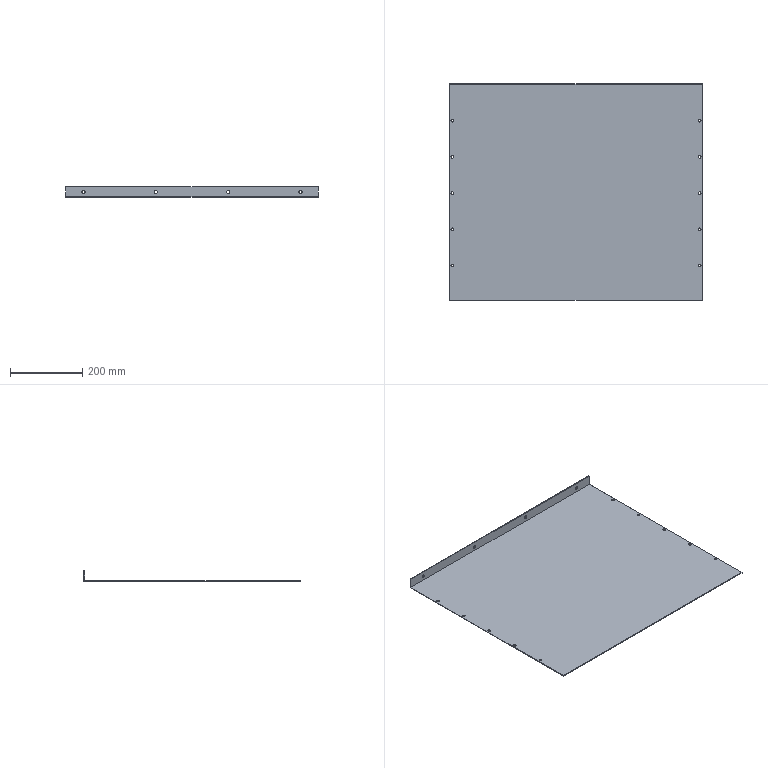Part | SolidWorks | features BaseBody 1 | 1 solid | 36 faces | box 699 x 599 x 30 mm | volume 1093155 mm3 | cylinder 28 | plane 8 | commonest cylinder face diameters 7.2 x20 9 x8
STEP:
#1=CARTESIAN_POINT('',(201.346,-3540.973,1409.971));
#2=VERTEX_POINT('',#1);
#3=CARTESIAN_POINT('',(208.546,-3540.973,1409.971));
#4=VERTEX_POINT('',#3);
#5=CARTESIAN_POINT('',(204.946,-3540.973,1409.971));
#6=DIRECTION('',(0.,0.,1.));
#7=DIRECTION('',(1.,0.,0.));
#8=AXIS2_PLACEMENT_3D('',#5,#6,#7);
#9=CIRCLE('',#8,3.6);
#10=EDGE_CURVE('',#2,#4,#9,.T.);
#11=ORIENTED_EDGE('',*,*,#10,.F.);
#12=CARTESIAN_POINT('',(201.346,-3540.973,1412.471));
#13=VERTEX_POINT('',#12);
#14=CARTESIAN_POINT('',(201.346,-3540.973,1411.476));
#15=DIRECTION('',(0.,0.,1.));
#16=VECTOR('',#15,1000.);
#17=LINE('',#14,#16);
#18=EDGE_CURVE('',#2,#13,#17,.T.);
#19=ORIENTED_EDGE('',*,*,#18,.T.);
#20=CARTESIAN_POINT('',(208.546,-3540.973,1412.471));
#21=VERTEX_POINT('',#20);
#22=CARTESIAN_POINT('',(204.946,-3540.973,1412.471));
#23=DIRECTION('',(0.,0.,-1.));
#24=DIRECTION('',(1.,0.,0.));
#25=AXIS2_PLACEMENT_3D('',#22,#23,#24);
#26=CIRCLE('',#25,3.6);
#27=EDGE_CURVE('',#21,#13,#26,.T.);
#28=ORIENTED_EDGE('',*,*,#27,.F.);
#29=CARTESIAN_POINT('',(208.546,-3540.973,1411.476));
#30=DIRECTION('',(0.,0.,1.));
#31=VECTOR('',#30,1000.);
#32=LINE('',#29,#31);
#33=EDGE_CURVE('',#4,#21,#32,.T.);
#34=ORIENTED_EDGE('',*,*,#33,.F.);
#35=EDGE_LOOP('',(#11,#19,#28,#34));
#36=FACE_OUTER_BOUND('',#35,.T.);
#37=CARTESIAN_POINT('',(204.946,-3540.973,1411.476));
#38=DIRECTION('',(0.,0.,1.));
#39=DIRECTION('',(1.,0.,0.));
#40=AXIS2_PLACEMENT_3D('',#37,#38,#39);
#41=CYLINDRICAL_SURFACE('',#40,3.6);
#42=ADVANCED_FACE('',(#36),#41,.F.);
#43=CARTESIAN_POINT('',(201.346,-3340.973,1409.971));
#44=VERTEX_POINT('',#43);
#45=CARTESIAN_POINT('',(208.546,-3340.973,1409.971));
#46=VERTEX_POINT('',#45);
#47=CARTESIAN_POINT('',(204.946,-3340.973,1409.971));
#48=DIRECTION('',(0.,0.,1.));
#49=DIRECTION('',(1.,0.,0.));
#50=AXIS2_PLACEMENT_3D('',#47,#48,#49);
#51=CIRCLE('',#50,3.6);
#52=EDGE_CURVE('',#44,#46,#51,.T.);
#53=ORIENTED_EDGE('',*,*,#52,.F.);
#54=CARTESIAN_POINT('',(201.346,-3340.973,1412.471));
#55=VERTEX_POINT('',#54);
#56=CARTESIAN_POINT('',(201.346,-3340.973,1411.476));
#57=DIRECTION('',(0.,0.,1.));
#58=VECTOR('',#57,1000.);
#59=LINE('',#56,#58);
#60=EDGE_CURVE('',#44,#55,#59,.T.);
#61=ORIENTED_EDGE('',*,*,#60,.T.);
#62=CARTESIAN_POINT('',(208.546,-3340.973,1412.471));
#63=VERTEX_POINT('',#62);
#64=CARTESIAN_POINT('',(204.946,-3340.973,1412.471));
#65=DIRECTION('',(0.,0.,-1.));
#66=DIRECTION('',(1.,0.,0.));
#67=AXIS2_PLACEMENT_3D('',#64,#65,#66);
#68=CIRCLE('',#67,3.6);
#69=EDGE_CURVE('',#63,#55,#68,.T.);
#70=ORIENTED_EDGE('',*,*,#69,.F.);
#71=CARTESIAN_POINT('',(208.546,-3340.973,1411.476));
#72=DIRECTION('',(0.,0.,1.));
#73=VECTOR('',#72,1000.);
#74=LINE('',#71,#73);
#75=EDGE_CURVE('',#46,#63,#74,.T.);
#76=ORIENTED_EDGE('',*,*,#75,.F.);
#77=EDGE_LOOP('',(#53,#61,#70,#76));
#78=FACE_OUTER_BOUND('',#77,.T.);
#79=CARTESIAN_POINT('',(204.946,-3340.973,1411.476));
#80=DIRECTION('',(0.,0.,1.));
#81=DIRECTION('',(1.,0.,0.));
#82=AXIS2_PLACEMENT_3D('',#79,#80,#81);
#83=CYLINDRICAL_SURFACE('',#82,3.6);
#84=ADVANCED_FACE('',(#78),#83,.F.);
#85=CARTESIAN_POINT('',(201.346,-3140.973,1409.971));
#86=VERTEX_POINT('',#85);
#87=CARTESIAN_POINT('',(208.546,-3140.973,1409.971));
#88=VERTEX_POINT('',#87);
#89=CARTESIAN_POINT('',(204.946,-3140.973,1409.971));
#90=DIRECTION('',(0.,0.,1.));
#91=DIRECTION('',(1.,0.,0.));
#92=AXIS2_PLACEMENT_3D('',#89,#90,#91);
#93=CIRCLE('',#92,3.6);
#94=EDGE_CURVE('',#86,#88,#93,.T.);
#95=ORIENTED_EDGE('',*,*,#94,.F.);
#96=CARTESIAN_POINT('',(201.346,-3140.973,1412.471));
#97=VERTEX_POINT('',#96);
#98=CARTESIAN_POINT('',(201.346,-3140.973,1411.476));
#99=DIRECTION('',(0.,0.,1.));
#100=VECTOR('',#99,1000.);
#101=LINE('',#98,#100);
#102=EDGE_CURVE('',#86,#97,#101,.T.);
#103=ORIENTED_EDGE('',*,*,#102,.T.);
#104=CARTESIAN_POINT('',(208.546,-3140.973,1412.471));
#105=VERTEX_POINT('',#104);
#106=CARTESIAN_POINT('',(204.946,-3140.973,1412.471));
#107=DIRECTION('',(0.,0.,-1.));
#108=DIRECTION('',(1.,0.,0.));
#109=AXIS2_PLACEMENT_3D('',#106,#107,#108);
#110=CIRCLE('',#109,3.6);
#111=EDGE_CURVE('',#105,#97,#110,.T.);
#112=ORIENTED_EDGE('',*,*,#111,.F.);
#113=CARTESIAN_POINT('',(208.546,-3140.973,1411.476));
#114=DIRECTION('',(0.,0.,1.));
#115=VECTOR('',#114,1000.);
#116=LINE('',#113,#115);
#117=EDGE_CURVE('',#88,#105,#116,.T.);
#118=ORIENTED_EDGE('',*,*,#117,.F.);
#119=EDGE_LOOP('',(#95,#103,#112,#118));
#120=FACE_OUTER_BOUND('',#119,.T.);
#121=CARTESIAN_POINT('',(204.946,-3140.973,1411.476));
#122=DIRECTION('',(0.,0.,1.));
#123=DIRECTION('',(1.,0.,0.));
#124=AXIS2_PLACEMENT_3D('',#121,#122,#123);
#125=CYLINDRICAL_SURFACE('',#124,3.6);
#126=ADVANCED_FACE('',(#120),#125,.F.);
#127=CARTESIAN_POINT('',(892.546,-3440.973,1412.471));
#128=VERTEX_POINT('',#127);
#129=CARTESIAN_POINT('',(885.346,-3440.973,1412.471));
#130=VERTEX_POINT('',#129);
#131=CARTESIAN_POINT('',(888.946,-3440.973,1412.471));
#132=DIRECTION('',(0.,0.,-1.));
#133=DIRECTION('',(-1.,0.,0.));
#134=AXIS2_PLACEMENT_3D('',#131,#132,#133);
#135=CIRCLE('',#134,3.6);
#136=EDGE_CURVE('',#128,#130,#135,.T.);
#137=ORIENTED_EDGE('',*,*,#136,.F.);
#138=CARTESIAN_POINT('',(892.546,-3440.973,1409.971));
#139=VERTEX_POINT('',#138);
#140=CARTESIAN_POINT('',(892.546,-3440.973,1411.476));
#141=DIRECTION('',(0.,0.,-1.));
#142=VECTOR('',#141,1000.);
#143=LINE('',#140,#142);
#144=EDGE_CURVE('',#128,#139,#143,.T.);
#145=ORIENTED_EDGE('',*,*,#144,.T.);
#146=CARTESIAN_POINT('',(885.346,-3440.973,1409.971));
#147=VERTEX_POINT('',#146);
#148=CARTESIAN_POINT('',(888.946,-3440.973,1409.971));
#149=DIRECTION('',(0.,0.,1.));
#150=DIRECTION('',(-1.,0.,0.));
#151=AXIS2_PLACEMENT_3D('',#148,#149,#150);
#152=CIRCLE('',#151,3.6);
#153=EDGE_CURVE('',#147,#139,#152,.T.);
#154=ORIENTED_EDGE('',*,*,#153,.F.);
#155=CARTESIAN_POINT('',(885.346,-3440.973,1411.476));
#156=DIRECTION('',(0.,0.,-1.));
#157=VECTOR('',#156,1000.);
#158=LINE('',#155,#157);
#159=EDGE_CURVE('',#130,#147,#158,.T.);
#160=ORIENTED_EDGE('',*,*,#159,.F.);
#161=EDGE_LOOP('',(#137,#145,#154,#160));
#162=FACE_OUTER_BOUND('',#161,.T.);
#163=CARTESIAN_POINT('',(888.946,-3440.973,1411.476));
#164=DIRECTION('',(0.,0.,-1.));
#165=DIRECTION('',(-1.,0.,0.));
#166=AXIS2_PLACEMENT_3D('',#163,#164,#165);
#167=CYLINDRICAL_SURFACE('',#166,3.6);
#168=ADVANCED_FACE('',(#162),#167,.F.);
#169=CARTESIAN_POINT('',(892.546,-3240.973,1412.471));
#170=VERTEX_POINT('',#169);
#171=CARTESIAN_POINT('',(885.346,-3240.973,1412.471));
#172=VERTEX_POINT('',#171);
#173=CARTESIAN_POINT('',(888.946,-3240.973,1412.471));
#174=DIRECTION('',(0.,0.,-1.));
#175=DIRECTION('',(-1.,0.,0.));
#176=AXIS2_PLACEMENT_3D('',#173,#174,#175);
#177=CIRCLE('',#176,3.6);
#178=EDGE_CURVE('',#170,#172,#177,.T.);
#179=ORIENTED_EDGE('',*,*,#178,.F.);
#180=CARTESIAN_POINT('',(892.546,-3240.973,1409.971));
#181=VERTEX_POINT('',#180);
#182=CARTESIAN_POINT('',(892.546,-3240.973,1411.476));
#183=DIRECTION('',(0.,0.,-1.));
#184=VECTOR('',#183,1000.);
#185=LINE('',#182,#184);
#186=EDGE_CURVE('',#170,#181,#185,.T.);
#187=ORIENTED_EDGE('',*,*,#186,.T.);
#188=CARTESIAN_POINT('',(885.346,-3240.973,1409.971));
#189=VERTEX_POINT('',#188);
#190=CARTESIAN_POINT('',(888.946,-3240.973,1409.971));
#191=DIRECTION('',(0.,0.,1.));
#192=DIRECTION('',(-1.,0.,0.));
#193=AXIS2_PLACEMENT_3D('',#190,#191,#192);
#194=CIRCLE('',#193,3.6);
#195=EDGE_CURVE('',#189,#181,#194,.T.);
#196=ORIENTED_EDGE('',*,*,#195,.F.);
#197=CARTESIAN_POINT('',(885.346,-3240.973,1411.476));
#198=DIRECTION('',(0.,0.,-1.));
#199=VECTOR('',#198,1000.);
#200=LINE('',#197,#199);
#201=EDGE_CURVE('',#172,#189,#200,.T.);
#202=ORIENTED_EDGE('',*,*,#201,.F.);
#203=EDGE_LOOP('',(#179,#187,#196,#202));
#204=FACE_OUTER_BOUND('',#203,.T.);
#205=CARTESIAN_POINT('',(888.946,-3240.973,1411.476));
#206=DIRECTION('',(0.,0.,-1.));
#207=DIRECTION('',(-1.,0.,0.));
#208=AXIS2_PLACEMENT_3D('',#205,#206,#207);
#209=CYLINDRICAL_SURFACE('',#208,3.6);
#210=ADVANCED_FACE('',(#204),#209,.F.);
#211=CARTESIAN_POINT('',(892.546,-3140.973,1412.471));
#212=VERTEX_POINT('',#211);
#213=CARTESIAN_POINT('',(885.346,-3140.973,1412.471));
#214=VERTEX_POINT('',#213);
#215=CARTESIAN_POINT('',(888.946,-3140.973,1412.471));
#216=DIRECTION('',(0.,0.,-1.));
#217=DIRECTION('',(-1.,0.,0.));
#218=AXIS2_PLACEMENT_3D('',#215,#216,#217);
#219=CIRCLE('',#218,3.6);
#220=EDGE_CURVE('',#212,#214,#219,.T.);
#221=ORIENTED_EDGE('',*,*,#220,.F.);
#222=CARTESIAN_POINT('',(892.546,-3140.973,1409.971));
#223=VERTEX_POINT('',#222);
#224=CARTESIAN_POINT('',(892.546,-3140.973,1411.476));
#225=DIRECTION('',(0.,0.,-1.));
#226=VECTOR('',#225,1000.);
#227=LINE('',#224,#226);
#228=EDGE_CURVE('',#212,#223,#227,.T.);
#229=ORIENTED_EDGE('',*,*,#228,.T.);
#230=CARTESIAN_POINT('',(885.346,-3140.973,1409.971));
#231=VERTEX_POINT('',#230);
#232=CARTESIAN_POINT('',(888.946,-3140.973,1409.971));
#233=DIRECTION('',(0.,0.,1.));
#234=DIRECTION('',(-1.,0.,0.));
#235=AXIS2_PLACEMENT_3D('',#232,#233,#234);
#236=CIRCLE('',#235,3.6);
#237=EDGE_CURVE('',#231,#223,#236,.T.);
#238=ORIENTED_EDGE('',*,*,#237,.F.);
#239=CARTESIAN_POINT('',(885.346,-3140.973,1411.476));
#240=DIRECTION('',(0.,0.,-1.));
#241=VECTOR('',#240,1000.);
#242=LINE('',#239,#241);
#243=EDGE_CURVE('',#214,#231,#242,.T.);
#244=ORIENTED_EDGE('',*,*,#243,.F.);
#245=EDGE_LOOP('',(#221,#229,#238,#244));
#246=FACE_OUTER_BOUND('',#245,.T.);
#247=CARTESIAN_POINT('',(888.946,-3140.973,1411.476));
#248=DIRECTION('',(0.,0.,-1.));
#249=DIRECTION('',(-1.,0.,0.));
#250=AXIS2_PLACEMENT_3D('',#247,#248,#249);
#251=CYLINDRICAL_SURFACE('',#250,3.6);
#252=ADVANCED_FACE('',(#246),#251,.F.);
#253=CARTESIAN_POINT('',(892.546,-3340.973,1412.471));
#254=VERTEX_POINT('',#253);
#255=CARTESIAN_POINT('',(885.346,-3340.973,1412.471));
#256=VERTEX_POINT('',#255);
#257=CARTESIAN_POINT('',(888.946,-3340.973,1412.471));
#258=DIRECTION('',(0.,0.,-1.));
#259=DIRECTION('',(-1.,0.,0.));
#260=AXIS2_PLACEMENT_3D('',#257,#258,#259);
#261=CIRCLE('',#260,3.6);
#262=EDGE_CURVE('',#254,#256,#261,.T.);
#263=ORIENTED_EDGE('',*,*,#262,.F.);
#264=CARTESIAN_POINT('',(892.546,-3340.973,1409.971));
#265=VERTEX_POINT('',#264);
#266=CARTESIAN_POINT('',(892.546,-3340.973,1411.476));
#267=DIRECTION('',(0.,0.,-1.));
#268=VECTOR('',#267,1000.);
#269=LINE('',#266,#268);
#270=EDGE_CURVE('',#254,#265,#269,.T.);
#271=ORIENTED_EDGE('',*,*,#270,.T.);
#272=CARTESIAN_POINT('',(885.346,-3340.973,1409.971));
#273=VERTEX_POINT('',#272);
#274=CARTESIAN_POINT('',(888.946,-3340.973,1409.971));
#275=DIRECTION('',(0.,0.,1.));
#276=DIRECTION('',(-1.,0.,0.));
#277=AXIS2_PLACEMENT_3D('',#274,#275,#276);
#278=CIRCLE('',#277,3.6);
#279=EDGE_CURVE('',#273,#265,#278,.T.);
#280=ORIENTED_EDGE('',*,*,#279,.F.);
#281=CARTESIAN_POINT('',(885.346,-3340.973,1411.476));
#282=DIRECTION('',(0.,0.,-1.));
#283=VECTOR('',#282,1000.);
#284=LINE('',#281,#283);
#285=EDGE_CURVE('',#256,#273,#284,.T.);
#286=ORIENTED_EDGE('',*,*,#285,.F.);
#287=EDGE_LOOP('',(#263,#271,#280,#286));
#288=FACE_OUTER_BOUND('',#287,.T.);
#289=CARTESIAN_POINT('',(888.946,-3340.973,1411.476));
#290=DIRECTION('',(0.,0.,-1.));
#291=DIRECTION('',(-1.,0.,0.));
#292=AXIS2_PLACEMENT_3D('',#289,#290,#291);
#293=CYLINDRICAL_SURFACE('',#292,3.6);
#294=ADVANCED_FACE('',(#288),#293,.F.);
#295=CARTESIAN_POINT('',(892.546,-3540.973,1412.471));
#296=VERTEX_POINT('',#295);
#297=CARTESIAN_POINT('',(885.346,-3540.973,1412.471));
#298=VERTEX_POINT('',#297);
#299=CARTESIAN_POINT('',(888.946,-3540.973,1412.471));
#300=DIRECTION('',(0.,0.,-1.));
#301=DIRECTION('',(-1.,0.,0.));
#302=AXIS2_PLACEMENT_3D('',#299,#300,#301);
#303=CIRCLE('',#302,3.6);
#304=EDGE_CURVE('',#296,#298,#303,.T.);
#305=ORIENTED_EDGE('',*,*,#304,.F.);
#306=CARTESIAN_POINT('',(892.546,-3540.973,1409.971));
#307=VERTEX_POINT('',#306);
#308=CARTESIAN_POINT('',(892.546,-3540.973,1411.476));
#309=DIRECTION('',(0.,0.,-1.));
#310=VECTOR('',#309,1000.);
#311=LINE('',#308,#310);
#312=EDGE_CURVE('',#296,#307,#311,.T.);
#313=ORIENTED_EDGE('',*,*,#312,.T.);
#314=CARTESIAN_POINT('',(885.346,-3540.973,1409.971));
#315=VERTEX_POINT('',#314);
#316=CARTESIAN_POINT('',(888.946,-3540.973,1409.971));
#317=DIRECTION('',(0.,0.,1.));
#318=DIRECTION('',(-1.,0.,0.));
#319=AXIS2_PLACEMENT_3D('',#316,#317,#318);
#320=CIRCLE('',#319,3.6);
#321=EDGE_CURVE('',#315,#307,#320,.T.);
#322=ORIENTED_EDGE('',*,*,#321,.F.);
#323=CARTESIAN_POINT('',(885.346,-3540.973,1411.476));
#324=DIRECTION('',(0.,0.,-1.));
#325=VECTOR('',#324,1000.);
#326=LINE('',#323,#325);
#327=EDGE_CURVE('',#298,#315,#326,.T.);
#328=ORIENTED_EDGE('',*,*,#327,.F.);
#329=EDGE_LOOP('',(#305,#313,#322,#328));
#330=FACE_OUTER_BOUND('',#329,.T.);
#331=CARTESIAN_POINT('',(888.946,-3540.973,1411.476));
#332=DIRECTION('',(0.,0.,-1.));
#333=DIRECTION('',(-1.,0.,0.));
#334=AXIS2_PLACEMENT_3D('',#331,#332,#333);
#335=CYLINDRICAL_SURFACE('',#334,3.6);
#336=ADVANCED_FACE('',(#330),#335,.F.);
#337=CARTESIAN_POINT('',(201.346,-3240.973,1409.971));
#338=VERTEX_POINT('',#337);
#339=CARTESIAN_POINT('',(208.546,-3240.973,1409.971));
#340=VERTEX_POINT('',#339);
#341=CARTESIAN_POINT('',(204.946,-3240.973,1409.971));
#342=DIRECTION('',(0.,0.,1.));
#343=DIRECTION('',(1.,0.,0.));
#344=AXIS2_PLACEMENT_3D('',#341,#342,#343);
#345=CIRCLE('',#344,3.6);
#346=EDGE_CURVE('',#338,#340,#345,.T.);
#347=ORIENTED_EDGE('',*,*,#346,.F.);
#348=CARTESIAN_POINT('',(201.346,-3240.973,1412.471));
#349=VERTEX_POINT('',#348);
#350=CARTESIAN_POINT('',(201.346,-3240.973,1411.476));
#351=DIRECTION('',(0.,0.,1.));
#352=VECTOR('',#351,1000.);
#353=LINE('',#350,#352);
#354=EDGE_CURVE('',#338,#349,#353,.T.);
#355=ORIENTED_EDGE('',*,*,#354,.T.);
#356=CARTESIAN_POINT('',(208.546,-3240.973,1412.471));
#357=VERTEX_POINT('',#356);
#358=CARTESIAN_POINT('',(204.946,-3240.973,1412.471));
#359=DIRECTION('',(0.,0.,-1.));
#360=DIRECTION('',(1.,0.,0.));
#361=AXIS2_PLACEMENT_3D('',#358,#359,#360);
#362=CIRCLE('',#361,3.6);
#363=EDGE_CURVE('',#357,#349,#362,.T.);
#364=ORIENTED_EDGE('',*,*,#363,.F.);
#365=CARTESIAN_POINT('',(208.546,-3240.973,1411.476));
#366=DIRECTION('',(0.,0.,1.));
#367=VECTOR('',#366,1000.);
#368=LINE('',#365,#367);
#369=EDGE_CURVE('',#340,#357,#368,.T.);
#370=ORIENTED_EDGE('',*,*,#369,.F.);
#371=EDGE_LOOP('',(#347,#355,#364,#370));
#372=FACE_OUTER_BOUND('',#371,.T.);
#373=CARTESIAN_POINT('',(204.946,-3240.973,1411.476));
#374=DIRECTION('',(0.,0.,1.));
#375=DIRECTION('',(1.,0.,0.));
#376=AXIS2_PLACEMENT_3D('',#373,#374,#375);
#377=CYLINDRICAL_SURFACE('',#376,3.6);
#378=ADVANCED_FACE('',(#372),#377,.F.);
#379=CARTESIAN_POINT('',(201.346,-3440.973,1409.971));
#380=VERTEX_POINT('',#379);
#381=CARTESIAN_POINT('',(208.546,-3440.973,1409.971));
#382=VERTEX_POINT('',#381);
#383=CARTESIAN_POINT('',(204.946,-3440.973,1409.971));
#384=DIRECTION('',(0.,0.,1.));
#385=DIRECTION('',(1.,0.,0.));
#386=AXIS2_PLACEMENT_3D('',#383,#384,#385);
#387=CIRCLE('',#386,3.6);
#388=EDGE_CURVE('',#380,#382,#387,.T.);
#389=ORIENTED_EDGE('',*,*,#388,.F.);
#390=CARTESIAN_POINT('',(201.346,-3440.973,1412.471));
#391=VERTEX_POINT('',#390);
#392=CARTESIAN_POINT('',(201.346,-3440.973,1411.476));
#393=DIRECTION('',(0.,0.,1.));
#394=VECTOR('',#393,1000.);
#395=LINE('',#392,#394);
#396=EDGE_CURVE('',#380,#391,#395,.T.);
#397=ORIENTED_EDGE('',*,*,#396,.T.);
#398=CARTESIAN_POINT('',(208.546,-3440.973,1412.471));
#399=VERTEX_POINT('',#398);
#400=CARTESIAN_POINT('',(204.946,-3440.973,1412.471));
#401=DIRECTION('',(0.,0.,-1.));
#402=DIRECTION('',(1.,0.,0.));
#403=AXIS2_PLACEMENT_3D('',#400,#401,#402);
#404=CIRCLE('',#403,3.6);
#405=EDGE_CURVE('',#399,#391,#404,.T.);
#406=ORIENTED_EDGE('',*,*,#405,.F.);
#407=CARTESIAN_POINT('',(208.546,-3440.973,1411.476));
#408=DIRECTION('',(0.,0.,1.));
#409=VECTOR('',#408,1000.);
#410=LINE('',#407,#409);
#411=EDGE_CURVE('',#382,#399,#410,.T.);
#412=ORIENTED_EDGE('',*,*,#411,.F.);
#413=EDGE_LOOP('',(#389,#397,#406,#412));
#414=FACE_OUTER_BOUND('',#413,.T.);
#415=CARTESIAN_POINT('',(204.946,-3440.973,1411.476));
#416=DIRECTION('',(0.,0.,1.));
#417=DIRECTION('',(1.,0.,0.));
#418=AXIS2_PLACEMENT_3D('',#415,#416,#417);
#419=CYLINDRICAL_SURFACE('',#418,3.6);
#420=ADVANCED_FACE('',(#414),#419,.F.);
#421=CARTESIAN_POINT('',(446.946,-3040.973,1420.471));
#422=VERTEX_POINT('',#421);
#423=CARTESIAN_POINT('',(446.946,-3040.973,1429.471));
#424=VERTEX_POINT('',#423);
#425=CARTESIAN_POINT('',(446.946,-3040.973,1424.971));
#426=DIRECTION('',(0.,1.,0.));
#427=DIRECTION('',(0.,0.,1.));
#428=AXIS2_PLACEMENT_3D('',#425,#426,#427);
#429=CIRCLE('',#428,4.5);
#430=EDGE_CURVE('',#422,#424,#429,.T.);
#431=ORIENTED_EDGE('',*,*,#430,.F.);
#432=CARTESIAN_POINT('',(446.946,-3038.473,1420.471));
#433=VERTEX_POINT('',#432);
#434=CARTESIAN_POINT('',(446.946,-3047.949,1420.471));
#435=DIRECTION('',(0.,1.,0.));
#436=VECTOR('',#435,1000.);
#437=LINE('',#434,#436);
#438=EDGE_CURVE('',#422,#433,#437,.T.);
#439=ORIENTED_EDGE('',*,*,#438,.T.);
#440=CARTESIAN_POINT('',(446.946,-3038.473,1429.471));
#441=VERTEX_POINT('',#440);
#442=CARTESIAN_POINT('',(446.946,-3038.473,1424.971));
#443=DIRECTION('',(0.,-1.,0.));
#444=DIRECTION('',(0.,0.,1.));
#445=AXIS2_PLACEMENT_3D('',#442,#443,#444);
#446=CIRCLE('',#445,4.5);
#447=EDGE_CURVE('',#441,#433,#446,.T.);
#448=ORIENTED_EDGE('',*,*,#447,.F.);
#449=CARTESIAN_POINT('',(446.946,-3047.949,1429.471));
#450=DIRECTION('',(0.,1.,0.));
#451=VECTOR('',#450,1000.);
#452=LINE('',#449,#451);
#453=EDGE_CURVE('',#424,#441,#452,.T.);
#454=ORIENTED_EDGE('',*,*,#453,.F.);
#455=EDGE_LOOP('',(#431,#439,#448,#454));
#456=FACE_OUTER_BOUND('',#455,.T.);
#457=CARTESIAN_POINT('',(446.946,-3047.949,1424.971));
#458=DIRECTION('',(0.,1.,0.));
#459=DIRECTION('',(0.,0.,1.));
#460=AXIS2_PLACEMENT_3D('',#457,#458,#459);
#461=CYLINDRICAL_SURFACE('',#460,4.5);
#462=ADVANCED_FACE('',(#456),#461,.F.);
#463=CARTESIAN_POINT('',(646.946,-3038.473,1429.471));
#464=VERTEX_POINT('',#463);
#465=CARTESIAN_POINT('',(646.946,-3038.473,1420.471));
#466=VERTEX_POINT('',#465);
#467=CARTESIAN_POINT('',(646.946,-3038.473,1424.971));
#468=DIRECTION('',(0.,-1.,0.));
#469=DIRECTION('',(0.,0.,-1.));
#470=AXIS2_PLACEMENT_3D('',#467,#468,#469);
#471=CIRCLE('',#470,4.5);
#472=EDGE_CURVE('',#464,#466,#471,.T.);
#473=ORIENTED_EDGE('',*,*,#472,.F.);
#474=CARTESIAN_POINT('',(646.946,-3040.973,1429.471));
#475=VERTEX_POINT('',#474);
#476=CARTESIAN_POINT('',(646.946,-3047.949,1429.471));
#477=DIRECTION('',(0.,-1.,0.));
#478=VECTOR('',#477,1000.);
#479=LINE('',#476,#478);
#480=EDGE_CURVE('',#464,#475,#479,.T.);
#481=ORIENTED_EDGE('',*,*,#480,.T.);
#482=CARTESIAN_POINT('',(646.946,-3040.973,1420.471));
#483=VERTEX_POINT('',#482);
#484=CARTESIAN_POINT('',(646.946,-3040.973,1424.971));
#485=DIRECTION('',(0.,1.,0.));
#486=DIRECTION('',(0.,0.,-1.));
#487=AXIS2_PLACEMENT_3D('',#484,#485,#486);
#488=CIRCLE('',#487,4.5);
#489=EDGE_CURVE('',#483,#475,#488,.T.);
#490=ORIENTED_EDGE('',*,*,#489,.F.);
#491=CARTESIAN_POINT('',(646.946,-3047.949,1420.471));
#492=DIRECTION('',(0.,-1.,0.));
#493=VECTOR('',#492,1000.);
#494=LINE('',#491,#493);
#495=EDGE_CURVE('',#466,#483,#494,.T.);
#496=ORIENTED_EDGE('',*,*,#495,.F.);
#497=EDGE_LOOP('',(#473,#481,#490,#496));
#498=FACE_OUTER_BOUND('',#497,.T.);
#499=CARTESIAN_POINT('',(646.946,-3047.949,1424.971));
#500=DIRECTION('',(0.,-1.,0.));
#501=DIRECTION('',(0.,0.,-1.));
#502=AXIS2_PLACEMENT_3D('',#499,#500,#501);
#503=CYLINDRICAL_SURFACE('',#502,4.5);
#504=ADVANCED_FACE('',(#498),#503,.F.);
#505=CARTESIAN_POINT('',(846.946,-3038.473,1429.471));
#506=VERTEX_POINT('',#505);
#507=CARTESIAN_POINT('',(846.946,-3038.473,1420.471));
#508=VERTEX_POINT('',#507);
#509=CARTESIAN_POINT('',(846.946,-3038.473,1424.971));
#510=DIRECTION('',(0.,-1.,0.));
#511=DIRECTION('',(0.,0.,-1.));
#512=AXIS2_PLACEMENT_3D('',#509,#510,#511);
#513=CIRCLE('',#512,4.5);
#514=EDGE_CURVE('',#506,#508,#513,.T.);
#515=ORIENTED_EDGE('',*,*,#514,.F.);
#516=CARTESIAN_POINT('',(846.946,-3040.973,1429.471));
#517=VERTEX_POINT('',#516);
#518=CARTESIAN_POINT('',(846.946,-3047.949,1429.471));
#519=DIRECTION('',(0.,-1.,0.));
#520=VECTOR('',#519,1000.);
#521=LINE('',#518,#520);
#522=EDGE_CURVE('',#506,#517,#521,.T.);
#523=ORIENTED_EDGE('',*,*,#522,.T.);
#524=CARTESIAN_POINT('',(846.946,-3040.973,1420.471));
#525=VERTEX_POINT('',#524);
#526=CARTESIAN_POINT('',(846.946,-3040.973,1424.971));
#527=DIRECTION('',(0.,1.,0.));
#528=DIRECTION('',(0.,0.,-1.));
#529=AXIS2_PLACEMENT_3D('',#526,#527,#528);
#530=CIRCLE('',#529,4.5);
#531=EDGE_CURVE('',#525,#517,#530,.T.);
#532=ORIENTED_EDGE('',*,*,#531,.F.);
#533=CARTESIAN_POINT('',(846.946,-3047.949,1420.471));
#534=DIRECTION('',(0.,-1.,0.));
#535=VECTOR('',#534,1000.);
#536=LINE('',#533,#535);
#537=EDGE_CURVE('',#508,#525,#536,.T.);
#538=ORIENTED_EDGE('',*,*,#537,.F.);
#539=EDGE_LOOP('',(#515,#523,#532,#538));
#540=FACE_OUTER_BOUND('',#539,.T.);
#541=CARTESIAN_POINT('',(846.946,-3047.949,1424.971));
#542=DIRECTION('',(0.,-1.,0.));
#543=DIRECTION('',(0.,0.,-1.));
#544=AXIS2_PLACEMENT_3D('',#541,#542,#543);
#545=CYLINDRICAL_SURFACE('',#544,4.5);
#546=ADVANCED_FACE('',(#540),#545,.F.);
#547=CARTESIAN_POINT('',(246.946,-3040.973,1420.471));
#548=VERTEX_POINT('',#547);
#549=CARTESIAN_POINT('',(246.946,-3040.973,1429.471));
#550=VERTEX_POINT('',#549);
#551=CARTESIAN_POINT('',(246.946,-3040.973,1424.971));
#552=DIRECTION('',(0.,1.,0.));
#553=DIRECTION('',(0.,0.,1.));
#554=AXIS2_PLACEMENT_3D('',#551,#552,#553);
#555=CIRCLE('',#554,4.5);
#556=EDGE_CURVE('',#548,#550,#555,.T.);
#557=ORIENTED_EDGE('',*,*,#556,.F.);
#558=CARTESIAN_POINT('',(246.946,-3038.473,1420.471));
#559=VERTEX_POINT('',#558);
#560=CARTESIAN_POINT('',(246.946,-3047.949,1420.471));
#561=DIRECTION('',(0.,1.,0.));
#562=VECTOR('',#561,1000.);
#563=LINE('',#560,#562);
#564=EDGE_CURVE('',#548,#559,#563,.T.);
#565=ORIENTED_EDGE('',*,*,#564,.T.);
#566=CARTESIAN_POINT('',(246.946,-3038.473,1429.471));
#567=VERTEX_POINT('',#566);
#568=CARTESIAN_POINT('',(246.946,-3038.473,1424.971));
#569=DIRECTION('',(0.,-1.,0.));
#570=DIRECTION('',(0.,0.,1.));
#571=AXIS2_PLACEMENT_3D('',#568,#569,#570);
#572=CIRCLE('',#571,4.5);
#573=EDGE_CURVE('',#567,#559,#572,.T.);
#574=ORIENTED_EDGE('',*,*,#573,.F.);
#575=CARTESIAN_POINT('',(246.946,-3047.949,1429.471));
#576=DIRECTION('',(0.,1.,0.));
#577=VECTOR('',#576,1000.);
#578=LINE('',#575,#577);
#579=EDGE_CURVE('',#550,#567,#578,.T.);
#580=ORIENTED_EDGE('',*,*,#579,.F.);
#581=EDGE_LOOP('',(#557,#565,#574,#580));
#582=FACE_OUTER_BOUND('',#581,.T.);
#583=CARTESIAN_POINT('',(246.946,-3047.949,1424.971));
#584=DIRECTION('',(0.,1.,0.));
#585=DIRECTION('',(0.,0.,1.));
#586=AXIS2_PLACEMENT_3D('',#583,#584,#585);
#587=CYLINDRICAL_SURFACE('',#586,4.5);
#588=ADVANCED_FACE('',(#582),#587,.F.);
#589=CARTESIAN_POINT('',(896.446,-3038.473,1409.971));
#590=VERTEX_POINT('',#589);
#591=CARTESIAN_POINT('',(896.446,-3637.473,1409.971));
#592=VERTEX_POINT('',#591);
#593=CARTESIAN_POINT('',(896.446,-3038.473,1409.971));
#594=DIRECTION('',(0.,-1.,0.));
#595=VECTOR('',#594,1000.);
#596=LINE('',#593,#595);
#597=EDGE_CURVE('',#590,#592,#596,.T.);
#598=ORIENTED_EDGE('',*,*,#597,.T.);
#599=CARTESIAN_POINT('',(197.446,-3637.473,1409.971));
#600=VERTEX_POINT('',#599);
#601=CARTESIAN_POINT('',(896.446,-3637.473,1409.971));
#602=DIRECTION('',(-1.,0.,0.));
#603=VECTOR('',#602,1000.);
#604=LINE('',#601,#603);
#605=EDGE_CURVE('',#592,#600,#604,.T.);
#606=ORIENTED_EDGE('',*,*,#605,.T.);
#607=CARTESIAN_POINT('',(197.446,-3038.473,1409.971));
#608=VERTEX_POINT('',#607);
#609=CARTESIAN_POINT('',(197.446,-3038.473,1409.971));
#610=DIRECTION('',(0.,1.,0.));
#611=VECTOR('',#610,1000.);
#612=LINE('',#609,#611);
#613=EDGE_CURVE('',#600,#608,#612,.T.);
#614=ORIENTED_EDGE('',*,*,#613,.T.);
#615=CARTESIAN_POINT('',(896.446,-3038.473,1409.971));
#616=DIRECTION('',(1.,0.,0.));
#617=VECTOR('',#616,1000.);
#618=LINE('',#615,#617);
#619=EDGE_CURVE('',#608,#590,#618,.T.);
#620=ORIENTED_EDGE('',*,*,#619,.T.);
#621=EDGE_LOOP('',(#598,#606,#614,#620));
#622=FACE_OUTER_BOUND('',#621,.T.);
#623=CARTESIAN_POINT('',(204.946,-3540.973,1409.971));
#624=DIRECTION('',(0.,0.,1.));
#625=DIRECTION('',(1.,0.,0.));
#626=AXIS2_PLACEMENT_3D('',#623,#624,#625);
#627=CIRCLE('',#626,3.6);
#628=EDGE_CURVE('',#4,#2,#627,.T.);
#629=ORIENTED_EDGE('',*,*,#628,.T.);
#630=ORIENTED_EDGE('',*,*,#10,.T.);
#631=EDGE_LOOP('',(#629,#630));
#632=FACE_BOUND('',#631,.T.);
#633=CARTESIAN_POINT('',(204.946,-3340.973,1409.971));
#634=DIRECTION('',(0.,0.,1.));
#635=DIRECTION('',(1.,0.,0.));
#636=AXIS2_PLACEMENT_3D('',#633,#634,#635);
#637=CIRCLE('',#636,3.6);
#638=EDGE_CURVE('',#46,#44,#637,.T.);
#639=ORIENTED_EDGE('',*,*,#638,.T.);
#640=ORIENTED_EDGE('',*,*,#52,.T.);
#641=EDGE_LOOP('',(#639,#640));
#642=FACE_BOUND('',#641,.T.);
#643=CARTESIAN_POINT('',(204.946,-3140.973,1409.971));
#644=DIRECTION('',(0.,0.,1.));
#645=DIRECTION('',(1.,0.,0.));
#646=AXIS2_PLACEMENT_3D('',#643,#644,#645);
#647=CIRCLE('',#646,3.6);
#648=EDGE_CURVE('',#88,#86,#647,.T.);
#649=ORIENTED_EDGE('',*,*,#648,.T.);
#650=ORIENTED_EDGE('',*,*,#94,.T.);
#651=EDGE_LOOP('',(#649,#650));
#652=FACE_BOUND('',#651,.T.);
#653=ORIENTED_EDGE('',*,*,#153,.T.);
#654=CARTESIAN_POINT('',(888.946,-3440.973,1409.971));
#655=DIRECTION('',(0.,0.,1.));
#656=DIRECTION('',(-1.,0.,0.));
#657=AXIS2_PLACEMENT_3D('',#654,#655,#656);
#658=CIRCLE('',#657,3.6);
#659=EDGE_CURVE('',#139,#147,#658,.T.);
#660=ORIENTED_EDGE('',*,*,#659,.T.);
#661=EDGE_LOOP('',(#653,#660));
#662=FACE_BOUND('',#661,.T.);
#663=ORIENTED_EDGE('',*,*,#195,.T.);
#664=CARTESIAN_POINT('',(888.946,-3240.973,1409.971));
#665=DIRECTION('',(0.,0.,1.));
#666=DIRECTION('',(-1.,0.,0.));
#667=AXIS2_PLACEMENT_3D('',#664,#665,#666);
#668=CIRCLE('',#667,3.6);
#669=EDGE_CURVE('',#181,#189,#668,.T.);
#670=ORIENTED_EDGE('',*,*,#669,.T.);
#671=EDGE_LOOP('',(#663,#670));
#672=FACE_BOUND('',#671,.T.);
#673=ORIENTED_EDGE('',*,*,#237,.T.);
#674=CARTESIAN_POINT('',(888.946,-3140.973,1409.971));
#675=DIRECTION('',(0.,0.,1.));
#676=DIRECTION('',(-1.,0.,0.));
#677=AXIS2_PLACEMENT_3D('',#674,#675,#676);
#678=CIRCLE('',#677,3.6);
#679=EDGE_CURVE('',#223,#231,#678,.T.);
#680=ORIENTED_EDGE('',*,*,#679,.T.);
#681=EDGE_LOOP('',(#673,#680));
#682=FACE_BOUND('',#681,.T.);
#683=ORIENTED_EDGE('',*,*,#279,.T.);
#684=CARTESIAN_POINT('',(888.946,-3340.973,1409.971));
#685=DIRECTION('',(0.,0.,1.));
#686=DIRECTION('',(-1.,0.,0.));
#687=AXIS2_PLACEMENT_3D('',#684,#685,#686);
#688=CIRCLE('',#687,3.6);
#689=EDGE_CURVE('',#265,#273,#688,.T.);
#690=ORIENTED_EDGE('',*,*,#689,.T.);
#691=EDGE_LOOP('',(#683,#690));
#692=FACE_BOUND('',#691,.T.);
#693=ORIENTED_EDGE('',*,*,#321,.T.);
#694=CARTESIAN_POINT('',(888.946,-3540.973,1409.971));
#695=DIRECTION('',(0.,0.,1.));
#696=DIRECTION('',(-1.,0.,0.));
#697=AXIS2_PLACEMENT_3D('',#694,#695,#696);
#698=CIRCLE('',#697,3.6);
#699=EDGE_CURVE('',#307,#315,#698,.T.);
#700=ORIENTED_EDGE('',*,*,#699,.T.);
#701=EDGE_LOOP('',(#693,#700));
#702=FACE_BOUND('',#701,.T.);
#703=CARTESIAN_POINT('',(204.946,-3240.973,1409.971));
#704=DIRECTION('',(0.,0.,1.));
#705=DIRECTION('',(1.,0.,0.));
#706=AXIS2_PLACEMENT_3D('',#703,#704,#705);
#707=CIRCLE('',#706,3.6);
#708=EDGE_CURVE('',#340,#338,#707,.T.);
#709=ORIENTED_EDGE('',*,*,#708,.T.);
#710=ORIENTED_EDGE('',*,*,#346,.T.);
#711=EDGE_LOOP('',(#709,#710));
#712=FACE_BOUND('',#711,.T.);
#713=CARTESIAN_POINT('',(204.946,-3440.973,1409.971));
#714=DIRECTION('',(0.,0.,1.));
#715=DIRECTION('',(1.,0.,0.));
#716=AXIS2_PLACEMENT_3D('',#713,#714,#715);
#717=CIRCLE('',#716,3.6);
#718=EDGE_CURVE('',#382,#380,#717,.T.);
#719=ORIENTED_EDGE('',*,*,#718,.T.);
#720=ORIENTED_EDGE('',*,*,#388,.T.);
#721=EDGE_LOOP('',(#719,#720));
#722=FACE_BOUND('',#721,.T.);
#723=CARTESIAN_POINT('',(896.446,-3038.473,1409.971));
#724=DIRECTION('',(0.,0.,-1.));
#725=DIRECTION('',(-1.,0.,0.));
#726=AXIS2_PLACEMENT_3D('',#723,#724,#725);
#727=PLANE('',#726);
#728=ADVANCED_FACE('',(#622,#632,#642,#652,#662,#672,#682,#692,#702,#712,#722),#727,.T.);
#729=CARTESIAN_POINT('',(896.446,-3637.473,1412.471));
#730=VERTEX_POINT('',#729);
#731=CARTESIAN_POINT('',(896.446,-3637.473,1409.971));
#732=DIRECTION('',(0.,0.,1.));
#733=VECTOR('',#732,1000.);
#734=LINE('',#731,#733);
#735=EDGE_CURVE('',#592,#730,#734,.T.);
#736=ORIENTED_EDGE('',*,*,#735,.T.);
#737=CARTESIAN_POINT('',(197.446,-3637.473,1412.471));
#738=VERTEX_POINT('',#737);
#739=CARTESIAN_POINT('',(896.446,-3637.473,1412.471));
#740=DIRECTION('',(-1.,0.,0.));
#741=VECTOR('',#740,1000.);
#742=LINE('',#739,#741);
#743=EDGE_CURVE('',#730,#738,#742,.T.);
#744=ORIENTED_EDGE('',*,*,#743,.T.);
#745=CARTESIAN_POINT('',(197.446,-3637.473,1409.971));
#746=DIRECTION('',(0.,0.,-1.));
#747=VECTOR('',#746,1000.);
#748=LINE('',#745,#747);
#749=EDGE_CURVE('',#738,#600,#748,.T.);
#750=ORIENTED_EDGE('',*,*,#749,.T.);
#751=ORIENTED_EDGE('',*,*,#605,.F.);
#752=EDGE_LOOP('',(#736,#744,#750,#751));
#753=FACE_OUTER_BOUND('',#752,.T.);
#754=CARTESIAN_POINT('',(896.446,-3637.473,1409.971));
#755=DIRECTION('',(0.,-1.,0.));
#756=DIRECTION('',(0.,0.,-1.));
#757=AXIS2_PLACEMENT_3D('',#754,#755,#756);
#758=PLANE('',#757);
#759=ADVANCED_FACE('',(#753),#758,.T.);
#760=ORIENTED_EDGE('',*,*,#735,.F.);
#761=ORIENTED_EDGE('',*,*,#597,.F.);
#762=CARTESIAN_POINT('',(896.446,-3038.473,1439.971));
#763=VERTEX_POINT('',#762);
#764=CARTESIAN_POINT('',(896.446,-3038.473,1411.717));
#765=DIRECTION('',(0.,0.,1.));
#766=VECTOR('',#765,1000.);
#767=LINE('',#764,#766);
#768=EDGE_CURVE('',#590,#763,#767,.T.);
#769=ORIENTED_EDGE('',*,*,#768,.T.);
#770=CARTESIAN_POINT('',(896.446,-3040.973,1439.971));
#771=VERTEX_POINT('',#770);
#772=CARTESIAN_POINT('',(896.446,-3327.219,1439.971));
#773=DIRECTION('',(0.,-1.,0.));
#774=VECTOR('',#773,1000.);
#775=LINE('',#772,#774);
#776=EDGE_CURVE('',#763,#771,#775,.T.);
#777=ORIENTED_EDGE('',*,*,#776,.T.);
#778=CARTESIAN_POINT('',(896.446,-3040.973,1412.471));
#779=VERTEX_POINT('',#778);
#780=CARTESIAN_POINT('',(896.446,-3040.973,1411.717));
#781=DIRECTION('',(0.,0.,-1.));
#782=VECTOR('',#781,1000.);
#783=LINE('',#780,#782);
#784=EDGE_CURVE('',#771,#779,#783,.T.);
#785=ORIENTED_EDGE('',*,*,#784,.T.);
#786=CARTESIAN_POINT('',(896.446,-3327.219,1412.471));
#787=DIRECTION('',(0.,-1.,0.));
#788=VECTOR('',#787,1000.);
#789=LINE('',#786,#788);
#790=EDGE_CURVE('',#779,#730,#789,.T.);
#791=ORIENTED_EDGE('',*,*,#790,.T.);
#792=EDGE_LOOP('',(#760,#761,#769,#777,#785,#791));
#793=FACE_OUTER_BOUND('',#792,.T.);
#794=CARTESIAN_POINT('',(896.446,-3327.219,1411.717));
#795=DIRECTION('',(1.,0.,0.));
#796=DIRECTION('',(0.,0.,-1.));
#797=AXIS2_PLACEMENT_3D('',#794,#795,#796);
#798=PLANE('',#797);
#799=ADVANCED_FACE('',(#793),#798,.T.);
#800=ORIENTED_EDGE('',*,*,#768,.F.);
#801=ORIENTED_EDGE('',*,*,#619,.F.);
#802=CARTESIAN_POINT('',(197.446,-3038.473,1439.971));
#803=VERTEX_POINT('',#802);
#804=CARTESIAN_POINT('',(197.446,-3038.473,1434.971));
#805=DIRECTION('',(0.,0.,1.));
#806=VECTOR('',#805,1000.);
#807=LINE('',#804,#806);
#808=EDGE_CURVE('',#608,#803,#807,.T.);
#809=ORIENTED_EDGE('',*,*,#808,.T.);
#810=CARTESIAN_POINT('',(896.446,-3038.473,1439.971));
#811=DIRECTION('',(1.,0.,0.));
#812=VECTOR('',#811,1000.);
#813=LINE('',#810,#812);
#814=EDGE_CURVE('',#803,#763,#813,.T.);
#815=ORIENTED_EDGE('',*,*,#814,.T.);
#816=EDGE_LOOP('',(#800,#801,#809,#815));
#817=FACE_OUTER_BOUND('',#816,.T.);
#818=ORIENTED_EDGE('',*,*,#447,.T.);
#819=CARTESIAN_POINT('',(446.946,-3038.473,1424.971));
#820=DIRECTION('',(0.,-1.,0.));
#821=DIRECTION('',(0.,0.,1.));
#822=AXIS2_PLACEMENT_3D('',#819,#820,#821);
#823=CIRCLE('',#822,4.5);
#824=EDGE_CURVE('',#433,#441,#823,.T.);
#825=ORIENTED_EDGE('',*,*,#824,.T.);
#826=EDGE_LOOP('',(#818,#825));
#827=FACE_BOUND('',#826,.T.);
#828=CARTESIAN_POINT('',(646.946,-3038.473,1424.971));
#829=DIRECTION('',(0.,-1.,0.));
#830=DIRECTION('',(0.,0.,-1.));
#831=AXIS2_PLACEMENT_3D('',#828,#829,#830);
#832=CIRCLE('',#831,4.5);
#833=EDGE_CURVE('',#466,#464,#832,.T.);
#834=ORIENTED_EDGE('',*,*,#833,.T.);
#835=ORIENTED_EDGE('',*,*,#472,.T.);
#836=EDGE_LOOP('',(#834,#835));
#837=FACE_BOUND('',#836,.T.);
#838=CARTESIAN_POINT('',(846.946,-3038.473,1424.971));
#839=DIRECTION('',(0.,-1.,0.));
#840=DIRECTION('',(0.,0.,-1.));
#841=AXIS2_PLACEMENT_3D('',#838,#839,#840);
#842=CIRCLE('',#841,4.5);
#843=EDGE_CURVE('',#508,#506,#842,.T.);
#844=ORIENTED_EDGE('',*,*,#843,.T.);
#845=ORIENTED_EDGE('',*,*,#514,.T.);
#846=EDGE_LOOP('',(#844,#845));
#847=FACE_BOUND('',#846,.T.);
#848=ORIENTED_EDGE('',*,*,#573,.T.);
#849=CARTESIAN_POINT('',(246.946,-3038.473,1424.971));
#850=DIRECTION('',(0.,-1.,0.));
#851=DIRECTION('',(0.,0.,1.));
#852=AXIS2_PLACEMENT_3D('',#849,#850,#851);
#853=CIRCLE('',#852,4.5);
#854=EDGE_CURVE('',#559,#567,#853,.T.);
#855=ORIENTED_EDGE('',*,*,#854,.T.);
#856=EDGE_LOOP('',(#848,#855));
#857=FACE_BOUND('',#856,.T.);
#858=CARTESIAN_POINT('',(896.446,-3038.473,1434.971));
#859=DIRECTION('',(0.,1.,0.));
#860=DIRECTION('',(0.,0.,1.));
#861=AXIS2_PLACEMENT_3D('',#858,#859,#860);
#862=PLANE('',#861);
#863=ADVANCED_FACE('',(#817,#827,#837,#847,#857),#862,.T.);
#864=ORIENTED_EDGE('',*,*,#749,.F.);
#865=CARTESIAN_POINT('',(197.446,-3040.973,1412.471));
#866=VERTEX_POINT('',#865);
#867=CARTESIAN_POINT('',(197.446,-3327.219,1412.471));
#868=DIRECTION('',(0.,-1.,0.));
#869=VECTOR('',#868,1000.);
#870=LINE('',#867,#869);
#871=EDGE_CURVE('',#866,#738,#870,.T.);
#872=ORIENTED_EDGE('',*,*,#871,.F.);
#873=CARTESIAN_POINT('',(197.446,-3040.973,1439.971));
#874=VERTEX_POINT('',#873);
#875=CARTESIAN_POINT('',(197.446,-3040.973,1416.717));
#876=DIRECTION('',(0.,0.,-1.));
#877=VECTOR('',#876,1000.);
#878=LINE('',#875,#877);
#879=EDGE_CURVE('',#874,#866,#878,.T.);
#880=ORIENTED_EDGE('',*,*,#879,.F.);
#881=CARTESIAN_POINT('',(197.446,-3327.219,1439.971));
#882=DIRECTION('',(0.,-1.,0.));
#883=VECTOR('',#882,1000.);
#884=LINE('',#881,#883);
#885=EDGE_CURVE('',#803,#874,#884,.T.);
#886=ORIENTED_EDGE('',*,*,#885,.F.);
#887=ORIENTED_EDGE('',*,*,#808,.F.);
#888=ORIENTED_EDGE('',*,*,#613,.F.);
#889=EDGE_LOOP('',(#864,#872,#880,#886,#887,#888));
#890=FACE_OUTER_BOUND('',#889,.T.);
#891=CARTESIAN_POINT('',(197.446,-3327.219,1416.717));
#892=DIRECTION('',(1.,0.,0.));
#893=DIRECTION('',(0.,0.,-1.));
#894=AXIS2_PLACEMENT_3D('',#891,#892,#893);
#895=PLANE('',#894);
#896=ADVANCED_FACE('',(#890),#895,.F.);
#897=ORIENTED_EDGE('',*,*,#18,.F.);
#898=ORIENTED_EDGE('',*,*,#628,.F.);
#899=ORIENTED_EDGE('',*,*,#33,.T.);
#900=CARTESIAN_POINT('',(204.946,-3540.973,1412.471));
#901=DIRECTION('',(0.,0.,-1.));
#902=DIRECTION('',(1.,0.,0.));
#903=AXIS2_PLACEMENT_3D('',#900,#901,#902);
#904=CIRCLE('',#903,3.6);
#905=EDGE_CURVE('',#13,#21,#904,.T.);
#906=ORIENTED_EDGE('',*,*,#905,.F.);
#907=EDGE_LOOP('',(#897,#898,#899,#906));
#908=FACE_OUTER_BOUND('',#907,.T.);
#909=CARTESIAN_POINT('',(204.946,-3540.973,1411.476));
#910=DIRECTION('',(0.,0.,1.));
#911=DIRECTION('',(1.,0.,0.));
#912=AXIS2_PLACEMENT_3D('',#909,#910,#911);
#913=CYLINDRICAL_SURFACE('',#912,3.6);
#914=ADVANCED_FACE('',(#908),#913,.F.);
#915=ORIENTED_EDGE('',*,*,#60,.F.);
#916=ORIENTED_EDGE('',*,*,#638,.F.);
#917=ORIENTED_EDGE('',*,*,#75,.T.);
#918=CARTESIAN_POINT('',(204.946,-3340.973,1412.471));
#919=DIRECTION('',(0.,0.,-1.));
#920=DIRECTION('',(1.,0.,0.));
#921=AXIS2_PLACEMENT_3D('',#918,#919,#920);
#922=CIRCLE('',#921,3.6);
#923=EDGE_CURVE('',#55,#63,#922,.T.);
#924=ORIENTED_EDGE('',*,*,#923,.F.);
#925=EDGE_LOOP('',(#915,#916,#917,#924));
#926=FACE_OUTER_BOUND('',#925,.T.);
#927=CARTESIAN_POINT('',(204.946,-3340.973,1411.476));
#928=DIRECTION('',(0.,0.,1.));
#929=DIRECTION('',(1.,0.,0.));
#930=AXIS2_PLACEMENT_3D('',#927,#928,#929);
#931=CYLINDRICAL_SURFACE('',#930,3.6);
#932=ADVANCED_FACE('',(#926),#931,.F.);
#933=ORIENTED_EDGE('',*,*,#102,.F.);
#934=ORIENTED_EDGE('',*,*,#648,.F.);
#935=ORIENTED_EDGE('',*,*,#117,.T.);
#936=CARTESIAN_POINT('',(204.946,-3140.973,1412.471));
#937=DIRECTION('',(0.,0.,-1.));
#938=DIRECTION('',(1.,0.,0.));
#939=AXIS2_PLACEMENT_3D('',#936,#937,#938);
#940=CIRCLE('',#939,3.6);
#941=EDGE_CURVE('',#97,#105,#940,.T.);
#942=ORIENTED_EDGE('',*,*,#941,.F.);
#943=EDGE_LOOP('',(#933,#934,#935,#942));
#944=FACE_OUTER_BOUND('',#943,.T.);
#945=CARTESIAN_POINT('',(204.946,-3140.973,1411.476));
#946=DIRECTION('',(0.,0.,1.));
#947=DIRECTION('',(1.,0.,0.));
#948=AXIS2_PLACEMENT_3D('',#945,#946,#947);
#949=CYLINDRICAL_SURFACE('',#948,3.6);
#950=ADVANCED_FACE('',(#944),#949,.F.);
#951=ORIENTED_EDGE('',*,*,#144,.F.);
#952=CARTESIAN_POINT('',(888.946,-3440.973,1412.471));
#953=DIRECTION('',(0.,0.,-1.));
#954=DIRECTION('',(-1.,0.,0.));
#955=AXIS2_PLACEMENT_3D('',#952,#953,#954);
#956=CIRCLE('',#955,3.6);
#957=EDGE_CURVE('',#130,#128,#956,.T.);
#958=ORIENTED_EDGE('',*,*,#957,.F.);
#959=ORIENTED_EDGE('',*,*,#159,.T.);
#960=ORIENTED_EDGE('',*,*,#659,.F.);
#961=EDGE_LOOP('',(#951,#958,#959,#960));
#962=FACE_OUTER_BOUND('',#961,.T.);
#963=CARTESIAN_POINT('',(888.946,-3440.973,1411.476));
#964=DIRECTION('',(0.,0.,-1.));
#965=DIRECTION('',(-1.,0.,0.));
#966=AXIS2_PLACEMENT_3D('',#963,#964,#965);
#967=CYLINDRICAL_SURFACE('',#966,3.6);
#968=ADVANCED_FACE('',(#962),#967,.F.);
#969=ORIENTED_EDGE('',*,*,#186,.F.);
#970=CARTESIAN_POINT('',(888.946,-3240.973,1412.471));
#971=DIRECTION('',(0.,0.,-1.));
#972=DIRECTION('',(-1.,0.,0.));
#973=AXIS2_PLACEMENT_3D('',#970,#971,#972);
#974=CIRCLE('',#973,3.6);
#975=EDGE_CURVE('',#172,#170,#974,.T.);
#976=ORIENTED_EDGE('',*,*,#975,.F.);
#977=ORIENTED_EDGE('',*,*,#201,.T.);
#978=ORIENTED_EDGE('',*,*,#669,.F.);
#979=EDGE_LOOP('',(#969,#976,#977,#978));
#980=FACE_OUTER_BOUND('',#979,.T.);
#981=CARTESIAN_POINT('',(888.946,-3240.973,1411.476));
#982=DIRECTION('',(0.,0.,-1.));
#983=DIRECTION('',(-1.,0.,0.));
#984=AXIS2_PLACEMENT_3D('',#981,#982,#983);
#985=CYLINDRICAL_SURFACE('',#984,3.6);
#986=ADVANCED_FACE('',(#980),#985,.F.);
#987=ORIENTED_EDGE('',*,*,#228,.F.);
#988=CARTESIAN_POINT('',(888.946,-3140.973,1412.471));
#989=DIRECTION('',(0.,0.,-1.));
#990=DIRECTION('',(-1.,0.,0.));
#991=AXIS2_PLACEMENT_3D('',#988,#989,#990);
#992=CIRCLE('',#991,3.6);
#993=EDGE_CURVE('',#214,#212,#992,.T.);
#994=ORIENTED_EDGE('',*,*,#993,.F.);
#995=ORIENTED_EDGE('',*,*,#243,.T.);
#996=ORIENTED_EDGE('',*,*,#679,.F.);
#997=EDGE_LOOP('',(#987,#994,#995,#996));
#998=FACE_OUTER_BOUND('',#997,.T.);
#999=CARTESIAN_POINT('',(888.946,-3140.973,1411.476));
#1000=DIRECTION('',(0.,0.,-1.));
#1001=DIRECTION('',(-1.,0.,0.));
#1002=AXIS2_PLACEMENT_3D('',#999,#1000,#1001);
#1003=CYLINDRICAL_SURFACE('',#1002,3.6);
#1004=ADVANCED_FACE('',(#998),#1003,.F.);
#1005=ORIENTED_EDGE('',*,*,#270,.F.);
#1006=CARTESIAN_POINT('',(888.946,-3340.973,1412.471));
#1007=DIRECTION('',(0.,0.,-1.));
#1008=DIRECTION('',(-1.,0.,0.));
#1009=AXIS2_PLACEMENT_3D('',#1006,#1007,#1008);
#1010=CIRCLE('',#1009,3.6);
#1011=EDGE_CURVE('',#256,#254,#1010,.T.);
#1012=ORIENTED_EDGE('',*,*,#1011,.F.);
#1013=ORIENTED_EDGE('',*,*,#285,.T.);
#1014=ORIENTED_EDGE('',*,*,#689,.F.);
#1015=EDGE_LOOP('',(#1005,#1012,#1013,#1014));
#1016=FACE_OUTER_BOUND('',#1015,.T.);
#1017=CARTESIAN_POINT('',(888.946,-3340.973,1411.476));
#1018=DIRECTION('',(0.,0.,-1.));
#1019=DIRECTION('',(-1.,0.,0.));
#1020=AXIS2_PLACEMENT_3D('',#1017,#1018,#1019);
#1021=CYLINDRICAL_SURFACE('',#1020,3.6);
#1022=ADVANCED_FACE('',(#1016),#1021,.F.);
#1023=ORIENTED_EDGE('',*,*,#312,.F.);
#1024=CARTESIAN_POINT('',(888.946,-3540.973,1412.471));
#1025=DIRECTION('',(0.,0.,-1.));
#1026=DIRECTION('',(-1.,0.,0.));
#1027=AXIS2_PLACEMENT_3D('',#1024,#1025,#1026);
#1028=CIRCLE('',#1027,3.6);
#1029=EDGE_CURVE('',#298,#296,#1028,.T.);
#1030=ORIENTED_EDGE('',*,*,#1029,.F.);
#1031=ORIENTED_EDGE('',*,*,#327,.T.);
#1032=ORIENTED_EDGE('',*,*,#699,.F.);
#1033=EDGE_LOOP('',(#1023,#1030,#1031,#1032));
#1034=FACE_OUTER_BOUND('',#1033,.T.);
#1035=CARTESIAN_POINT('',(888.946,-3540.973,1411.476));
#1036=DIRECTION('',(0.,0.,-1.));
#1037=DIRECTION('',(-1.,0.,0.));
#1038=AXIS2_PLACEMENT_3D('',#1035,#1036,#1037);
#1039=CYLINDRICAL_SURFACE('',#1038,3.6);
#1040=ADVANCED_FACE('',(#1034),#1039,.F.);
#1041=ORIENTED_EDGE('',*,*,#354,.F.);
#1042=ORIENTED_EDGE('',*,*,#708,.F.);
#1043=ORIENTED_EDGE('',*,*,#369,.T.);
#1044=CARTESIAN_POINT('',(204.946,-3240.973,1412.471));
#1045=DIRECTION('',(0.,0.,-1.));
#1046=DIRECTION('',(1.,0.,0.));
#1047=AXIS2_PLACEMENT_3D('',#1044,#1045,#1046);
#1048=CIRCLE('',#1047,3.6);
#1049=EDGE_CURVE('',#349,#357,#1048,.T.);
#1050=ORIENTED_EDGE('',*,*,#1049,.F.);
#1051=EDGE_LOOP('',(#1041,#1042,#1043,#1050));
#1052=FACE_OUTER_BOUND('',#1051,.T.);
#1053=CARTESIAN_POINT('',(204.946,-3240.973,1411.476));
#1054=DIRECTION('',(0.,0.,1.));
#1055=DIRECTION('',(1.,0.,0.));
#1056=AXIS2_PLACEMENT_3D('',#1053,#1054,#1055);
#1057=CYLINDRICAL_SURFACE('',#1056,3.6);
#1058=ADVANCED_FACE('',(#1052),#1057,.F.);
#1059=ORIENTED_EDGE('',*,*,#396,.F.);
#1060=ORIENTED_EDGE('',*,*,#718,.F.);
#1061=ORIENTED_EDGE('',*,*,#411,.T.);
#1062=CARTESIAN_POINT('',(204.946,-3440.973,1412.471));
#1063=DIRECTION('',(0.,0.,-1.));
#1064=DIRECTION('',(1.,0.,0.));
#1065=AXIS2_PLACEMENT_3D('',#1062,#1063,#1064);
#1066=CIRCLE('',#1065,3.6);
#1067=EDGE_CURVE('',#391,#399,#1066,.T.);
#1068=ORIENTED_EDGE('',*,*,#1067,.F.);
#1069=EDGE_LOOP('',(#1059,#1060,#1061,#1068));
#1070=FACE_OUTER_BOUND('',#1069,.T.);
#1071=CARTESIAN_POINT('',(204.946,-3440.973,1411.476));
#1072=DIRECTION('',(0.,0.,1.));
#1073=DIRECTION('',(1.,0.,0.));
#1074=AXIS2_PLACEMENT_3D('',#1071,#1072,#1073);
#1075=CYLINDRICAL_SURFACE('',#1074,3.6);
#1076=ADVANCED_FACE('',(#1070),#1075,.F.);
#1077=ORIENTED_EDGE('',*,*,#790,.F.);
#1078=CARTESIAN_POINT('',(896.446,-3040.973,1412.471));
#1079=DIRECTION('',(-1.,0.,0.));
#1080=VECTOR('',#1079,1000.);
#1081=LINE('',#1078,#1080);
#1082=EDGE_CURVE('',#779,#866,#1081,.T.);
#1083=ORIENTED_EDGE('',*,*,#1082,.T.);
#1084=ORIENTED_EDGE('',*,*,#871,.T.);
#1085=ORIENTED_EDGE('',*,*,#743,.F.);
#1086=EDGE_LOOP('',(#1077,#1083,#1084,#1085));
#1087=FACE_OUTER_BOUND('',#1086,.T.);
#1088=ORIENTED_EDGE('',*,*,#27,.T.);
#1089=ORIENTED_EDGE('',*,*,#905,.T.);
#1090=EDGE_LOOP('',(#1088,#1089));
#1091=FACE_BOUND('',#1090,.T.);
#1092=ORIENTED_EDGE('',*,*,#69,.T.);
#1093=ORIENTED_EDGE('',*,*,#923,.T.);
#1094=EDGE_LOOP('',(#1092,#1093));
#1095=FACE_BOUND('',#1094,.T.);
#1096=ORIENTED_EDGE('',*,*,#111,.T.);
#1097=ORIENTED_EDGE('',*,*,#941,.T.);
#1098=EDGE_LOOP('',(#1096,#1097));
#1099=FACE_BOUND('',#1098,.T.);
#1100=ORIENTED_EDGE('',*,*,#957,.T.);
#1101=ORIENTED_EDGE('',*,*,#136,.T.);
#1102=EDGE_LOOP('',(#1100,#1101));
#1103=FACE_BOUND('',#1102,.T.);
#1104=ORIENTED_EDGE('',*,*,#975,.T.);
#1105=ORIENTED_EDGE('',*,*,#178,.T.);
#1106=EDGE_LOOP('',(#1104,#1105));
#1107=FACE_BOUND('',#1106,.T.);
#1108=ORIENTED_EDGE('',*,*,#993,.T.);
#1109=ORIENTED_EDGE('',*,*,#220,.T.);
#1110=EDGE_LOOP('',(#1108,#1109));
#1111=FACE_BOUND('',#1110,.T.);
#1112=ORIENTED_EDGE('',*,*,#1011,.T.);
#1113=ORIENTED_EDGE('',*,*,#262,.T.);
#1114=EDGE_LOOP('',(#1112,#1113));
#1115=FACE_BOUND('',#1114,.T.);
#1116=ORIENTED_EDGE('',*,*,#1029,.T.);
#1117=ORIENTED_EDGE('',*,*,#304,.T.);
#1118=EDGE_LOOP('',(#1116,#1117));
#1119=FACE_BOUND('',#1118,.T.);
#1120=ORIENTED_EDGE('',*,*,#363,.T.);
#1121=ORIENTED_EDGE('',*,*,#1049,.T.);
#1122=EDGE_LOOP('',(#1120,#1121));
#1123=FACE_BOUND('',#1122,.T.);
#1124=ORIENTED_EDGE('',*,*,#405,.T.);
#1125=ORIENTED_EDGE('',*,*,#1067,.T.);
#1126=EDGE_LOOP('',(#1124,#1125));
#1127=FACE_BOUND('',#1126,.T.);
#1128=CARTESIAN_POINT('',(896.446,-3637.473,1412.471));
#1129=DIRECTION('',(0.,0.,1.));
#1130=DIRECTION('',(1.,0.,0.));
#1131=AXIS2_PLACEMENT_3D('',#1128,#1129,#1130);
#1132=PLANE('',#1131);
#1133=ADVANCED_FACE('',(#1087,#1091,#1095,#1099,#1103,#1107,#1111,#1115,#1119,#1123,#1127),#1132,.T.);
#1134=ORIENTED_EDGE('',*,*,#784,.F.);
#1135=CARTESIAN_POINT('',(896.446,-3040.973,1439.971));
#1136=DIRECTION('',(-1.,0.,0.));
#1137=VECTOR('',#1136,1000.);
#1138=LINE('',#1135,#1137);
#1139=EDGE_CURVE('',#771,#874,#1138,.T.);
#1140=ORIENTED_EDGE('',*,*,#1139,.T.);
#1141=ORIENTED_EDGE('',*,*,#879,.T.);
#1142=ORIENTED_EDGE('',*,*,#1082,.F.);
#1143=EDGE_LOOP('',(#1134,#1140,#1141,#1142));
#1144=FACE_OUTER_BOUND('',#1143,.T.);
#1145=CARTESIAN_POINT('',(446.946,-3040.973,1424.971));
#1146=DIRECTION('',(0.,1.,0.));
#1147=DIRECTION('',(0.,0.,1.));
#1148=AXIS2_PLACEMENT_3D('',#1145,#1146,#1147);
#1149=CIRCLE('',#1148,4.5);
#1150=EDGE_CURVE('',#424,#422,#1149,.T.);
#1151=ORIENTED_EDGE('',*,*,#1150,.T.);
#1152=ORIENTED_EDGE('',*,*,#430,.T.);
#1153=EDGE_LOOP('',(#1151,#1152));
#1154=FACE_BOUND('',#1153,.T.);
#1155=ORIENTED_EDGE('',*,*,#489,.T.);
#1156=CARTESIAN_POINT('',(646.946,-3040.973,1424.971));
#1157=DIRECTION('',(0.,1.,0.));
#1158=DIRECTION('',(0.,0.,-1.));
#1159=AXIS2_PLACEMENT_3D('',#1156,#1157,#1158);
#1160=CIRCLE('',#1159,4.5);
#1161=EDGE_CURVE('',#475,#483,#1160,.T.);
#1162=ORIENTED_EDGE('',*,*,#1161,.T.);
#1163=EDGE_LOOP('',(#1155,#1162));
#1164=FACE_BOUND('',#1163,.T.);
#1165=ORIENTED_EDGE('',*,*,#531,.T.);
#1166=CARTESIAN_POINT('',(846.946,-3040.973,1424.971));
#1167=DIRECTION('',(0.,1.,0.));
#1168=DIRECTION('',(0.,0.,-1.));
#1169=AXIS2_PLACEMENT_3D('',#1166,#1167,#1168);
#1170=CIRCLE('',#1169,4.5);
#1171=EDGE_CURVE('',#517,#525,#1170,.T.);
#1172=ORIENTED_EDGE('',*,*,#1171,.T.);
#1173=EDGE_LOOP('',(#1165,#1172));
#1174=FACE_BOUND('',#1173,.T.);
#1175=CARTESIAN_POINT('',(246.946,-3040.973,1424.971));
#1176=DIRECTION('',(0.,1.,0.));
#1177=DIRECTION('',(0.,0.,1.));
#1178=AXIS2_PLACEMENT_3D('',#1175,#1176,#1177);
#1179=CIRCLE('',#1178,4.5);
#1180=EDGE_CURVE('',#550,#548,#1179,.T.);
#1181=ORIENTED_EDGE('',*,*,#1180,.T.);
#1182=ORIENTED_EDGE('',*,*,#556,.T.);
#1183=EDGE_LOOP('',(#1181,#1182));
#1184=FACE_BOUND('',#1183,.T.);
#1185=CARTESIAN_POINT('',(896.446,-3040.973,1412.471));
#1186=DIRECTION('',(0.,-1.,0.));
#1187=DIRECTION('',(0.,0.,-1.));
#1188=AXIS2_PLACEMENT_3D('',#1185,#1186,#1187);
#1189=PLANE('',#1188);
#1190=ADVANCED_FACE('',(#1144,#1154,#1164,#1174,#1184),#1189,.T.);
#1191=ORIENTED_EDGE('',*,*,#776,.F.);
#1192=ORIENTED_EDGE('',*,*,#814,.F.);
#1193=ORIENTED_EDGE('',*,*,#885,.T.);
#1194=ORIENTED_EDGE('',*,*,#1139,.F.);
#1195=EDGE_LOOP('',(#1191,#1192,#1193,#1194));
#1196=FACE_OUTER_BOUND('',#1195,.T.);
#1197=CARTESIAN_POINT('',(896.446,-3040.973,1439.971));
#1198=DIRECTION('',(0.,0.,1.));
#1199=DIRECTION('',(1.,0.,0.));
#1200=AXIS2_PLACEMENT_3D('',#1197,#1198,#1199);
#1201=PLANE('',#1200);
#1202=ADVANCED_FACE('',(#1196),#1201,.T.);
#1203=ORIENTED_EDGE('',*,*,#438,.F.);
#1204=ORIENTED_EDGE('',*,*,#1150,.F.);
#1205=ORIENTED_EDGE('',*,*,#453,.T.);
#1206=ORIENTED_EDGE('',*,*,#824,.F.);
#1207=EDGE_LOOP('',(#1203,#1204,#1205,#1206));
#1208=FACE_OUTER_BOUND('',#1207,.T.);
#1209=CARTESIAN_POINT('',(446.946,-3047.949,1424.971));
#1210=DIRECTION('',(0.,1.,0.));
#1211=DIRECTION('',(0.,0.,1.));
#1212=AXIS2_PLACEMENT_3D('',#1209,#1210,#1211);
#1213=CYLINDRICAL_SURFACE('',#1212,4.5);
#1214=ADVANCED_FACE('',(#1208),#1213,.F.);
#1215=ORIENTED_EDGE('',*,*,#480,.F.);
#1216=ORIENTED_EDGE('',*,*,#833,.F.);
#1217=ORIENTED_EDGE('',*,*,#495,.T.);
#1218=ORIENTED_EDGE('',*,*,#1161,.F.);
#1219=EDGE_LOOP('',(#1215,#1216,#1217,#1218));
#1220=FACE_OUTER_BOUND('',#1219,.T.);
#1221=CARTESIAN_POINT('',(646.946,-3047.949,1424.971));
#1222=DIRECTION('',(0.,-1.,0.));
#1223=DIRECTION('',(0.,0.,-1.));
#1224=AXIS2_PLACEMENT_3D('',#1221,#1222,#1223);
#1225=CYLINDRICAL_SURFACE('',#1224,4.5);
#1226=ADVANCED_FACE('',(#1220),#1225,.F.);
#1227=ORIENTED_EDGE('',*,*,#522,.F.);
#1228=ORIENTED_EDGE('',*,*,#843,.F.);
#1229=ORIENTED_EDGE('',*,*,#537,.T.);
#1230=ORIENTED_EDGE('',*,*,#1171,.F.);
#1231=EDGE_LOOP('',(#1227,#1228,#1229,#1230));
#1232=FACE_OUTER_BOUND('',#1231,.T.);
#1233=CARTESIAN_POINT('',(846.946,-3047.949,1424.971));
#1234=DIRECTION('',(0.,-1.,0.));
#1235=DIRECTION('',(0.,0.,-1.));
#1236=AXIS2_PLACEMENT_3D('',#1233,#1234,#1235);
#1237=CYLINDRICAL_SURFACE('',#1236,4.5);
#1238=ADVANCED_FACE('',(#1232),#1237,.F.);
#1239=ORIENTED_EDGE('',*,*,#564,.F.);
#1240=ORIENTED_EDGE('',*,*,#1180,.F.);
#1241=ORIENTED_EDGE('',*,*,#579,.T.);
#1242=ORIENTED_EDGE('',*,*,#854,.F.);
#1243=EDGE_LOOP('',(#1239,#1240,#1241,#1242));
#1244=FACE_OUTER_BOUND('',#1243,.T.);
#1245=CARTESIAN_POINT('',(246.946,-3047.949,1424.971));
#1246=DIRECTION('',(0.,1.,0.));
#1247=DIRECTION('',(0.,0.,1.));
#1248=AXIS2_PLACEMENT_3D('',#1245,#1246,#1247);
#1249=CYLINDRICAL_SURFACE('',#1248,4.5);
#1250=ADVANCED_FACE('',(#1244),#1249,.F.);
#1251=CLOSED_SHELL('',(#42,#84,#126,#168,#210,#252,#294,#336,#378,#420,#462,#504,#546,#588,#728,#759,#799,#863,#896,#914,#932,#950,#968,#986,#1004,#1022,#1040,#1058,#1076,#1133,#1190,#1202,#1214,#1226,#1238,#1250));
#1252=MANIFOLD_SOLID_BREP('',#1251);
#1253=CARTESIAN_POINT('',(0.,0.,0.));
#1254=DIRECTION('',(0.,0.,1.));
#1255=DIRECTION('',(1.,0.,0.));
#1256=AXIS2_PLACEMENT_3D('',#1253,#1254,#1255);
#1257=(LENGTH_UNIT()NAMED_UNIT(*)SI_UNIT(.MILLI.,.METRE.));
#1258=UNCERTAINTY_MEASURE_WITH_UNIT(LENGTH_MEASURE(0.00001),#1257,'','');
#1259=(NAMED_UNIT(*)PLANE_ANGLE_UNIT()SI_UNIT($,.RADIAN.));
#1260=(NAMED_UNIT(*)SI_UNIT($,.STERADIAN.)SOLID_ANGLE_UNIT());
#1261=(GEOMETRIC_REPRESENTATION_CONTEXT(3)GLOBAL_UNCERTAINTY_ASSIGNED_CONTEXT((#1258))GLOBAL_UNIT_ASSIGNED_CONTEXT((#1257,#1259,#1260))REPRESENTATION_CONTEXT('',''));
#1262=ADVANCED_BREP_SHAPE_REPRESENTATION('',(#1252,#1256),#1261);